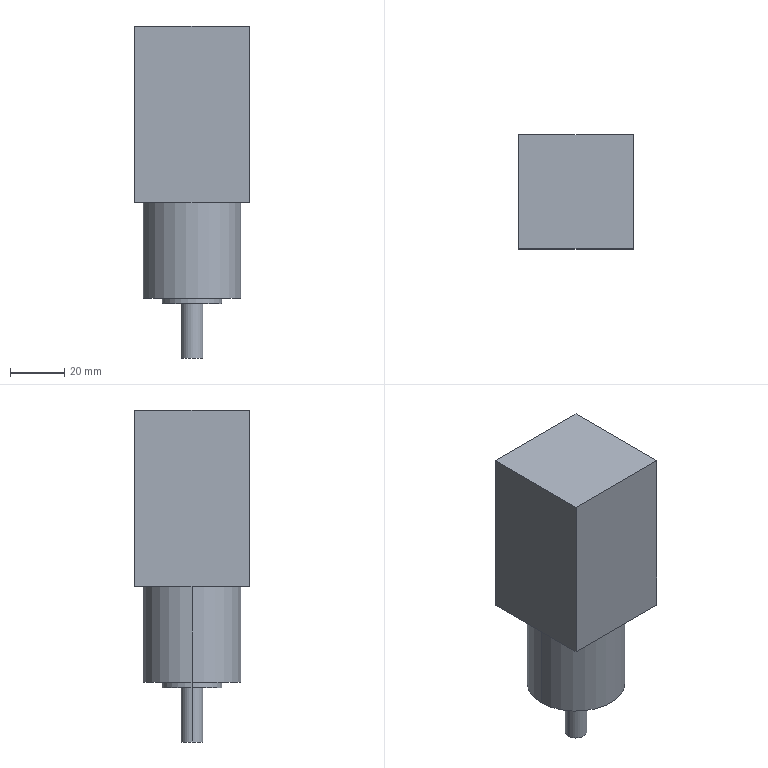Part | NX | features BREP 1 | 1 solid | 15 faces | box 42 x 42 x 122 mm | volume 152051 mm3 | plane 9 | cylinder 6 | commonest cylinder face diameters 8 x2 22 x2 36 x2
STEP:
#1=CARTESIAN_POINT('',(4.,0.,-57.));
#2=VERTEX_POINT('',#1);
#3=CARTESIAN_POINT('',(-4.,0.,-57.));
#4=VERTEX_POINT('',#3);
#5=CARTESIAN_POINT('',(0.,0.,-57.));
#6=DIRECTION('',(0.,0.,-1.));
#7=DIRECTION('',(-1.,0.,0.));
#8=AXIS2_PLACEMENT_3D('',#5,#6,#7);
#9=CIRCLE('',#8,4.);
#10=EDGE_CURVE('',#2,#4,#9,.T.);
#11=ORIENTED_EDGE('',*,*,#10,.T.);
#12=CARTESIAN_POINT('',(0.,0.,-57.));
#13=DIRECTION('',(0.,0.,-1.));
#14=DIRECTION('',(-1.,0.,0.));
#15=AXIS2_PLACEMENT_3D('',#12,#13,#14);
#16=CIRCLE('',#15,4.);
#17=EDGE_CURVE('',#4,#2,#16,.T.);
#18=ORIENTED_EDGE('',*,*,#17,.T.);
#19=EDGE_LOOP('',(#11,#18));
#20=FACE_BOUND('',#19,.T.);
#21=CARTESIAN_POINT('',(0.,0.,-57.));
#22=DIRECTION('',(0.,0.,-1.));
#23=DIRECTION('',(-1.,0.,0.));
#24=AXIS2_PLACEMENT_3D('',#21,#22,#23);
#25=PLANE('',#24);
#26=ADVANCED_FACE('',(#20),#25,.T.);
#27=CARTESIAN_POINT('',(-4.,0.,-37.));
#28=VERTEX_POINT('',#27);
#29=CARTESIAN_POINT('',(-4.,0.,-57.));
#30=DIRECTION('',(0.,0.,1.));
#31=VECTOR('',#30,1000.);
#32=LINE('',#29,#31);
#33=EDGE_CURVE('',#28,#4,#32,.F.);
#34=ORIENTED_EDGE('',*,*,#33,.T.);
#35=ORIENTED_EDGE('',*,*,#10,.F.);
#36=CARTESIAN_POINT('',(4.,0.,-37.));
#37=VERTEX_POINT('',#36);
#38=CARTESIAN_POINT('',(4.,0.,-57.));
#39=DIRECTION('',(0.,0.,1.));
#40=VECTOR('',#39,1000.);
#41=LINE('',#38,#40);
#42=EDGE_CURVE('',#37,#2,#41,.F.);
#43=ORIENTED_EDGE('',*,*,#42,.F.);
#44=CARTESIAN_POINT('',(0.,0.,-37.));
#45=DIRECTION('',(0.,0.,-1.));
#46=DIRECTION('',(-1.,0.,0.));
#47=AXIS2_PLACEMENT_3D('',#44,#45,#46);
#48=CIRCLE('',#47,4.);
#49=EDGE_CURVE('',#37,#28,#48,.T.);
#50=ORIENTED_EDGE('',*,*,#49,.T.);
#51=EDGE_LOOP('',(#34,#35,#43,#50));
#52=FACE_BOUND('',#51,.T.);
#53=CARTESIAN_POINT('',(0.,0.,-57.));
#54=DIRECTION('',(0.,0.,1.));
#55=DIRECTION('',(1.,0.,0.));
#56=AXIS2_PLACEMENT_3D('',#53,#54,#55);
#57=CYLINDRICAL_SURFACE('',#56,4.);
#58=ADVANCED_FACE('',(#52),#57,.T.);
#59=CARTESIAN_POINT('',(11.,0.,-37.));
#60=VERTEX_POINT('',#59);
#61=CARTESIAN_POINT('',(-11.,0.,-37.));
#62=VERTEX_POINT('',#61);
#63=CARTESIAN_POINT('',(0.,0.,-37.));
#64=DIRECTION('',(0.,0.,-1.));
#65=DIRECTION('',(-1.,0.,0.));
#66=AXIS2_PLACEMENT_3D('',#63,#64,#65);
#67=CIRCLE('',#66,11.);
#68=EDGE_CURVE('',#60,#62,#67,.T.);
#69=ORIENTED_EDGE('',*,*,#68,.T.);
#70=CARTESIAN_POINT('',(0.,0.,-37.));
#71=DIRECTION('',(0.,0.,-1.));
#72=DIRECTION('',(-1.,0.,0.));
#73=AXIS2_PLACEMENT_3D('',#70,#71,#72);
#74=CIRCLE('',#73,11.);
#75=EDGE_CURVE('',#62,#60,#74,.T.);
#76=ORIENTED_EDGE('',*,*,#75,.T.);
#77=EDGE_LOOP('',(#69,#76));
#78=FACE_BOUND('',#77,.T.);
#79=ORIENTED_EDGE('',*,*,#49,.F.);
#80=CARTESIAN_POINT('',(0.,0.,-37.));
#81=DIRECTION('',(0.,0.,-1.));
#82=DIRECTION('',(-1.,0.,0.));
#83=AXIS2_PLACEMENT_3D('',#80,#81,#82);
#84=CIRCLE('',#83,4.);
#85=EDGE_CURVE('',#28,#37,#84,.T.);
#86=ORIENTED_EDGE('',*,*,#85,.F.);
#87=EDGE_LOOP('',(#79,#86));
#88=FACE_BOUND('',#87,.T.);
#89=CARTESIAN_POINT('',(0.,0.,-37.));
#90=DIRECTION('',(0.,0.,-1.));
#91=DIRECTION('',(-1.,0.,0.));
#92=AXIS2_PLACEMENT_3D('',#89,#90,#91);
#93=PLANE('',#92);
#94=ADVANCED_FACE('',(#78,#88),#93,.T.);
#95=CARTESIAN_POINT('',(-11.,0.,-35.));
#96=VERTEX_POINT('',#95);
#97=CARTESIAN_POINT('',(-11.,0.,-37.));
#98=DIRECTION('',(0.,0.,1.));
#99=VECTOR('',#98,1000.);
#100=LINE('',#97,#99);
#101=EDGE_CURVE('',#96,#62,#100,.F.);
#102=ORIENTED_EDGE('',*,*,#101,.T.);
#103=ORIENTED_EDGE('',*,*,#68,.F.);
#104=CARTESIAN_POINT('',(11.,0.,-35.));
#105=VERTEX_POINT('',#104);
#106=CARTESIAN_POINT('',(11.,0.,-37.));
#107=DIRECTION('',(0.,0.,1.));
#108=VECTOR('',#107,1000.);
#109=LINE('',#106,#108);
#110=EDGE_CURVE('',#105,#60,#109,.F.);
#111=ORIENTED_EDGE('',*,*,#110,.F.);
#112=CARTESIAN_POINT('',(0.,0.,-35.));
#113=DIRECTION('',(0.,0.,-1.));
#114=DIRECTION('',(-1.,0.,0.));
#115=AXIS2_PLACEMENT_3D('',#112,#113,#114);
#116=CIRCLE('',#115,11.);
#117=EDGE_CURVE('',#105,#96,#116,.T.);
#118=ORIENTED_EDGE('',*,*,#117,.T.);
#119=EDGE_LOOP('',(#102,#103,#111,#118));
#120=FACE_BOUND('',#119,.T.);
#121=CARTESIAN_POINT('',(0.,0.,-37.));
#122=DIRECTION('',(0.,0.,1.));
#123=DIRECTION('',(1.,0.,0.));
#124=AXIS2_PLACEMENT_3D('',#121,#122,#123);
#125=CYLINDRICAL_SURFACE('',#124,11.);
#126=ADVANCED_FACE('',(#120),#125,.T.);
#127=CARTESIAN_POINT('',(18.,0.,-35.));
#128=VERTEX_POINT('',#127);
#129=CARTESIAN_POINT('',(-18.,0.,-35.));
#130=VERTEX_POINT('',#129);
#131=CARTESIAN_POINT('',(0.,0.,-35.));
#132=DIRECTION('',(0.,0.,-1.));
#133=DIRECTION('',(-1.,0.,0.));
#134=AXIS2_PLACEMENT_3D('',#131,#132,#133);
#135=CIRCLE('',#134,18.);
#136=EDGE_CURVE('',#128,#130,#135,.T.);
#137=ORIENTED_EDGE('',*,*,#136,.T.);
#138=CARTESIAN_POINT('',(0.,0.,-35.));
#139=DIRECTION('',(0.,0.,-1.));
#140=DIRECTION('',(-1.,0.,0.));
#141=AXIS2_PLACEMENT_3D('',#138,#139,#140);
#142=CIRCLE('',#141,18.);
#143=EDGE_CURVE('',#130,#128,#142,.T.);
#144=ORIENTED_EDGE('',*,*,#143,.T.);
#145=EDGE_LOOP('',(#137,#144));
#146=FACE_BOUND('',#145,.T.);
#147=ORIENTED_EDGE('',*,*,#117,.F.);
#148=CARTESIAN_POINT('',(0.,0.,-35.));
#149=DIRECTION('',(0.,0.,-1.));
#150=DIRECTION('',(-1.,0.,0.));
#151=AXIS2_PLACEMENT_3D('',#148,#149,#150);
#152=CIRCLE('',#151,11.);
#153=EDGE_CURVE('',#96,#105,#152,.T.);
#154=ORIENTED_EDGE('',*,*,#153,.F.);
#155=EDGE_LOOP('',(#147,#154));
#156=FACE_BOUND('',#155,.T.);
#157=CARTESIAN_POINT('',(0.,0.,-35.));
#158=DIRECTION('',(0.,0.,-1.));
#159=DIRECTION('',(-1.,0.,0.));
#160=AXIS2_PLACEMENT_3D('',#157,#158,#159);
#161=PLANE('',#160);
#162=ADVANCED_FACE('',(#146,#156),#161,.T.);
#163=CARTESIAN_POINT('',(-18.,0.,0.));
#164=VERTEX_POINT('',#163);
#165=CARTESIAN_POINT('',(-18.,0.,-35.));
#166=DIRECTION('',(0.,0.,1.));
#167=VECTOR('',#166,1000.);
#168=LINE('',#165,#167);
#169=EDGE_CURVE('',#164,#130,#168,.F.);
#170=ORIENTED_EDGE('',*,*,#169,.T.);
#171=ORIENTED_EDGE('',*,*,#136,.F.);
#172=CARTESIAN_POINT('',(18.,0.,0.));
#173=VERTEX_POINT('',#172);
#174=CARTESIAN_POINT('',(18.,0.,-35.));
#175=DIRECTION('',(0.,0.,1.));
#176=VECTOR('',#175,1000.);
#177=LINE('',#174,#176);
#178=EDGE_CURVE('',#173,#128,#177,.F.);
#179=ORIENTED_EDGE('',*,*,#178,.F.);
#180=CARTESIAN_POINT('',(0.,0.,0.));
#181=DIRECTION('',(0.,0.,-1.));
#182=DIRECTION('',(-1.,0.,0.));
#183=AXIS2_PLACEMENT_3D('',#180,#181,#182);
#184=CIRCLE('',#183,18.);
#185=EDGE_CURVE('',#173,#164,#184,.T.);
#186=ORIENTED_EDGE('',*,*,#185,.T.);
#187=EDGE_LOOP('',(#170,#171,#179,#186));
#188=FACE_BOUND('',#187,.T.);
#189=CARTESIAN_POINT('',(0.,0.,-35.));
#190=DIRECTION('',(0.,0.,1.));
#191=DIRECTION('',(1.,0.,0.));
#192=AXIS2_PLACEMENT_3D('',#189,#190,#191);
#193=CYLINDRICAL_SURFACE('',#192,18.);
#194=ADVANCED_FACE('',(#188),#193,.T.);
#195=CARTESIAN_POINT('',(21.,-21.,0.));
#196=VERTEX_POINT('',#195);
#197=CARTESIAN_POINT('',(21.,21.,0.));
#198=VERTEX_POINT('',#197);
#199=CARTESIAN_POINT('',(21.,-21.,0.));
#200=DIRECTION('',(0.,1.,0.));
#201=VECTOR('',#200,1000.);
#202=LINE('',#199,#201);
#203=EDGE_CURVE('',#196,#198,#202,.T.);
#204=ORIENTED_EDGE('',*,*,#203,.F.);
#205=CARTESIAN_POINT('',(-21.,-21.,0.));
#206=VERTEX_POINT('',#205);
#207=CARTESIAN_POINT('',(-21.,-21.,0.));
#208=DIRECTION('',(1.,0.,0.));
#209=VECTOR('',#208,1000.);
#210=LINE('',#207,#209);
#211=EDGE_CURVE('',#206,#196,#210,.T.);
#212=ORIENTED_EDGE('',*,*,#211,.F.);
#213=CARTESIAN_POINT('',(-21.,21.,0.));
#214=VERTEX_POINT('',#213);
#215=CARTESIAN_POINT('',(-21.,-21.,0.));
#216=DIRECTION('',(0.,-1.,0.));
#217=VECTOR('',#216,1000.);
#218=LINE('',#215,#217);
#219=EDGE_CURVE('',#214,#206,#218,.T.);
#220=ORIENTED_EDGE('',*,*,#219,.F.);
#221=CARTESIAN_POINT('',(-21.,21.,0.));
#222=DIRECTION('',(-1.,0.,0.));
#223=VECTOR('',#222,1000.);
#224=LINE('',#221,#223);
#225=EDGE_CURVE('',#198,#214,#224,.T.);
#226=ORIENTED_EDGE('',*,*,#225,.F.);
#227=EDGE_LOOP('',(#204,#212,#220,#226));
#228=FACE_BOUND('',#227,.T.);
#229=ORIENTED_EDGE('',*,*,#185,.F.);
#230=CARTESIAN_POINT('',(0.,0.,0.));
#231=DIRECTION('',(0.,0.,-1.));
#232=DIRECTION('',(-1.,0.,0.));
#233=AXIS2_PLACEMENT_3D('',#230,#231,#232);
#234=CIRCLE('',#233,18.);
#235=EDGE_CURVE('',#164,#173,#234,.T.);
#236=ORIENTED_EDGE('',*,*,#235,.F.);
#237=EDGE_LOOP('',(#229,#236));
#238=FACE_BOUND('',#237,.T.);
#239=CARTESIAN_POINT('',(0.,0.,0.));
#240=DIRECTION('',(0.,0.,-1.));
#241=DIRECTION('',(-1.,0.,0.));
#242=AXIS2_PLACEMENT_3D('',#239,#240,#241);
#243=PLANE('',#242);
#244=ADVANCED_FACE('',(#228,#238),#243,.T.);
#245=CARTESIAN_POINT('',(21.,-21.,65.));
#246=VERTEX_POINT('',#245);
#247=CARTESIAN_POINT('',(21.,21.,65.));
#248=VERTEX_POINT('',#247);
#249=CARTESIAN_POINT('',(21.,-21.,65.));
#250=DIRECTION('',(0.,1.,0.));
#251=VECTOR('',#250,1000.);
#252=LINE('',#249,#251);
#253=EDGE_CURVE('',#246,#248,#252,.T.);
#254=ORIENTED_EDGE('',*,*,#253,.T.);
#255=CARTESIAN_POINT('',(-21.,21.,65.));
#256=VERTEX_POINT('',#255);
#257=CARTESIAN_POINT('',(-21.,21.,65.));
#258=DIRECTION('',(-1.,0.,0.));
#259=VECTOR('',#258,1000.);
#260=LINE('',#257,#259);
#261=EDGE_CURVE('',#248,#256,#260,.T.);
#262=ORIENTED_EDGE('',*,*,#261,.T.);
#263=CARTESIAN_POINT('',(-21.,-21.,65.));
#264=VERTEX_POINT('',#263);
#265=CARTESIAN_POINT('',(-21.,-21.,65.));
#266=DIRECTION('',(0.,-1.,0.));
#267=VECTOR('',#266,1000.);
#268=LINE('',#265,#267);
#269=EDGE_CURVE('',#256,#264,#268,.T.);
#270=ORIENTED_EDGE('',*,*,#269,.T.);
#271=CARTESIAN_POINT('',(-21.,-21.,65.));
#272=DIRECTION('',(1.,0.,0.));
#273=VECTOR('',#272,1000.);
#274=LINE('',#271,#273);
#275=EDGE_CURVE('',#264,#246,#274,.T.);
#276=ORIENTED_EDGE('',*,*,#275,.T.);
#277=EDGE_LOOP('',(#254,#262,#270,#276));
#278=FACE_BOUND('',#277,.T.);
#279=CARTESIAN_POINT('',(0.,0.,65.));
#280=DIRECTION('',(0.,0.,-1.));
#281=DIRECTION('',(-1.,0.,0.));
#282=AXIS2_PLACEMENT_3D('',#279,#280,#281);
#283=PLANE('',#282);
#284=ADVANCED_FACE('',(#278),#283,.F.);
#285=ORIENTED_EDGE('',*,*,#211,.T.);
#286=CARTESIAN_POINT('',(21.,-21.,65.));
#287=DIRECTION('',(0.,0.,-1.));
#288=VECTOR('',#287,1000.);
#289=LINE('',#286,#288);
#290=EDGE_CURVE('',#246,#196,#289,.T.);
#291=ORIENTED_EDGE('',*,*,#290,.F.);
#292=ORIENTED_EDGE('',*,*,#275,.F.);
#293=CARTESIAN_POINT('',(-21.,-21.,65.));
#294=DIRECTION('',(0.,0.,-1.));
#295=VECTOR('',#294,1000.);
#296=LINE('',#293,#295);
#297=EDGE_CURVE('',#264,#206,#296,.T.);
#298=ORIENTED_EDGE('',*,*,#297,.T.);
#299=EDGE_LOOP('',(#285,#291,#292,#298));
#300=FACE_BOUND('',#299,.T.);
#301=CARTESIAN_POINT('',(-21.,-21.,65.));
#302=DIRECTION('',(0.,1.,0.));
#303=DIRECTION('',(0.,0.,1.));
#304=AXIS2_PLACEMENT_3D('',#301,#302,#303);
#305=PLANE('',#304);
#306=ADVANCED_FACE('',(#300),#305,.F.);
#307=ORIENTED_EDGE('',*,*,#219,.T.);
#308=ORIENTED_EDGE('',*,*,#297,.F.);
#309=ORIENTED_EDGE('',*,*,#269,.F.);
#310=CARTESIAN_POINT('',(-21.,21.,65.));
#311=DIRECTION('',(0.,0.,-1.));
#312=VECTOR('',#311,1000.);
#313=LINE('',#310,#312);
#314=EDGE_CURVE('',#256,#214,#313,.T.);
#315=ORIENTED_EDGE('',*,*,#314,.T.);
#316=EDGE_LOOP('',(#307,#308,#309,#315));
#317=FACE_BOUND('',#316,.T.);
#318=CARTESIAN_POINT('',(-21.,-21.,65.));
#319=DIRECTION('',(1.,0.,0.));
#320=DIRECTION('',(0.,0.,-1.));
#321=AXIS2_PLACEMENT_3D('',#318,#319,#320);
#322=PLANE('',#321);
#323=ADVANCED_FACE('',(#317),#322,.F.);
#324=ORIENTED_EDGE('',*,*,#225,.T.);
#325=ORIENTED_EDGE('',*,*,#314,.F.);
#326=ORIENTED_EDGE('',*,*,#261,.F.);
#327=CARTESIAN_POINT('',(21.,21.,65.));
#328=DIRECTION('',(0.,0.,-1.));
#329=VECTOR('',#328,1000.);
#330=LINE('',#327,#329);
#331=EDGE_CURVE('',#248,#198,#330,.T.);
#332=ORIENTED_EDGE('',*,*,#331,.T.);
#333=EDGE_LOOP('',(#324,#325,#326,#332));
#334=FACE_BOUND('',#333,.T.);
#335=CARTESIAN_POINT('',(-21.,21.,65.));
#336=DIRECTION('',(0.,-1.,0.));
#337=DIRECTION('',(0.,0.,-1.));
#338=AXIS2_PLACEMENT_3D('',#335,#336,#337);
#339=PLANE('',#338);
#340=ADVANCED_FACE('',(#334),#339,.F.);
#341=ORIENTED_EDGE('',*,*,#203,.T.);
#342=ORIENTED_EDGE('',*,*,#331,.F.);
#343=ORIENTED_EDGE('',*,*,#253,.F.);
#344=ORIENTED_EDGE('',*,*,#290,.T.);
#345=EDGE_LOOP('',(#341,#342,#343,#344));
#346=FACE_BOUND('',#345,.T.);
#347=CARTESIAN_POINT('',(21.,-21.,65.));
#348=DIRECTION('',(-1.,0.,0.));
#349=DIRECTION('',(0.,0.,1.));
#350=AXIS2_PLACEMENT_3D('',#347,#348,#349);
#351=PLANE('',#350);
#352=ADVANCED_FACE('',(#346),#351,.F.);
#353=ORIENTED_EDGE('',*,*,#143,.F.);
#354=ORIENTED_EDGE('',*,*,#169,.F.);
#355=ORIENTED_EDGE('',*,*,#235,.T.);
#356=ORIENTED_EDGE('',*,*,#178,.T.);
#357=EDGE_LOOP('',(#353,#354,#355,#356));
#358=FACE_BOUND('',#357,.T.);
#359=CARTESIAN_POINT('',(0.,0.,-35.));
#360=DIRECTION('',(0.,0.,1.));
#361=DIRECTION('',(1.,0.,0.));
#362=AXIS2_PLACEMENT_3D('',#359,#360,#361);
#363=CYLINDRICAL_SURFACE('',#362,18.);
#364=ADVANCED_FACE('',(#358),#363,.T.);
#365=ORIENTED_EDGE('',*,*,#75,.F.);
#366=ORIENTED_EDGE('',*,*,#101,.F.);
#367=ORIENTED_EDGE('',*,*,#153,.T.);
#368=ORIENTED_EDGE('',*,*,#110,.T.);
#369=EDGE_LOOP('',(#365,#366,#367,#368));
#370=FACE_BOUND('',#369,.T.);
#371=CARTESIAN_POINT('',(0.,0.,-37.));
#372=DIRECTION('',(0.,0.,1.));
#373=DIRECTION('',(1.,0.,0.));
#374=AXIS2_PLACEMENT_3D('',#371,#372,#373);
#375=CYLINDRICAL_SURFACE('',#374,11.);
#376=ADVANCED_FACE('',(#370),#375,.T.);
#377=ORIENTED_EDGE('',*,*,#17,.F.);
#378=ORIENTED_EDGE('',*,*,#33,.F.);
#379=ORIENTED_EDGE('',*,*,#85,.T.);
#380=ORIENTED_EDGE('',*,*,#42,.T.);
#381=EDGE_LOOP('',(#377,#378,#379,#380));
#382=FACE_BOUND('',#381,.T.);
#383=CARTESIAN_POINT('',(0.,0.,-57.));
#384=DIRECTION('',(0.,0.,1.));
#385=DIRECTION('',(1.,0.,0.));
#386=AXIS2_PLACEMENT_3D('',#383,#384,#385);
#387=CYLINDRICAL_SURFACE('',#386,4.);
#388=ADVANCED_FACE('',(#382),#387,.T.);
#389=CLOSED_SHELL('',(#26,#58,#94,#126,#162,#194,#244,#284,#306,#323,#340,#352,#364,#376,#388));
#390=MANIFOLD_SOLID_BREP('',#389);
#391=(LENGTH_UNIT()NAMED_UNIT(*)SI_UNIT(.MILLI.,.METRE.));
#392=UNCERTAINTY_MEASURE_WITH_UNIT(LENGTH_MEASURE(0.00001),#391,'','');
#393=(NAMED_UNIT(*)PLANE_ANGLE_UNIT()SI_UNIT($,.RADIAN.));
#394=(NAMED_UNIT(*)SI_UNIT($,.STERADIAN.)SOLID_ANGLE_UNIT());
#395=(GEOMETRIC_REPRESENTATION_CONTEXT(3)GLOBAL_UNCERTAINTY_ASSIGNED_CONTEXT((#392))GLOBAL_UNIT_ASSIGNED_CONTEXT((#391,#393,#394))REPRESENTATION_CONTEXT('',''));
#396=ADVANCED_BREP_SHAPE_REPRESENTATION('',(#390),#395);